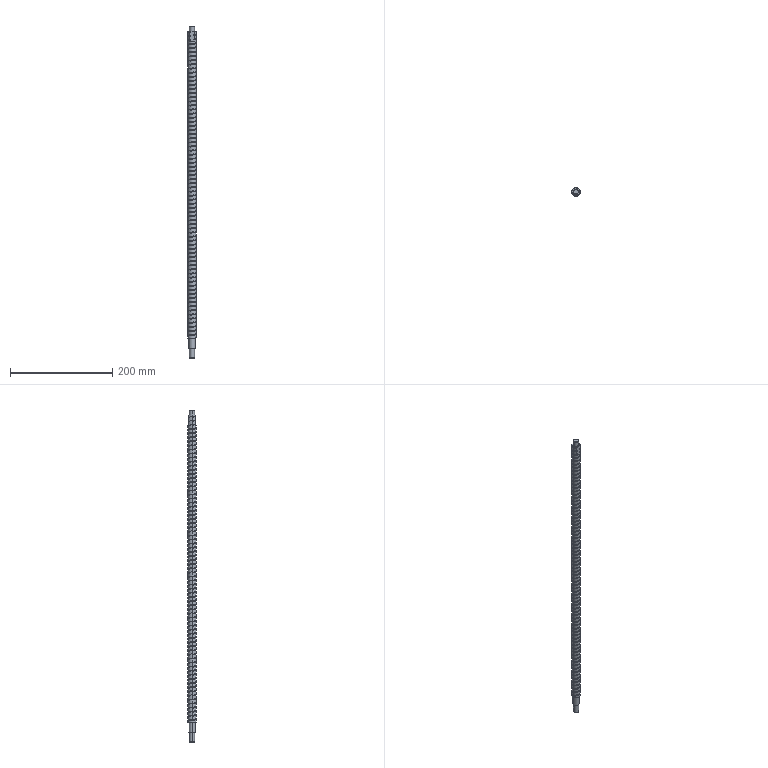Part | STEP file | -01 screw pair SFUR1604-648 | 1 solid | 187 faces | box 16 x 16 x 648 mm | volume 118967 mm3 | cylinder 165 | plane 12 | spline 6 | cone 4 | commonest cylinder face diameters 16 x155 3 x4 10 x4 12 x2